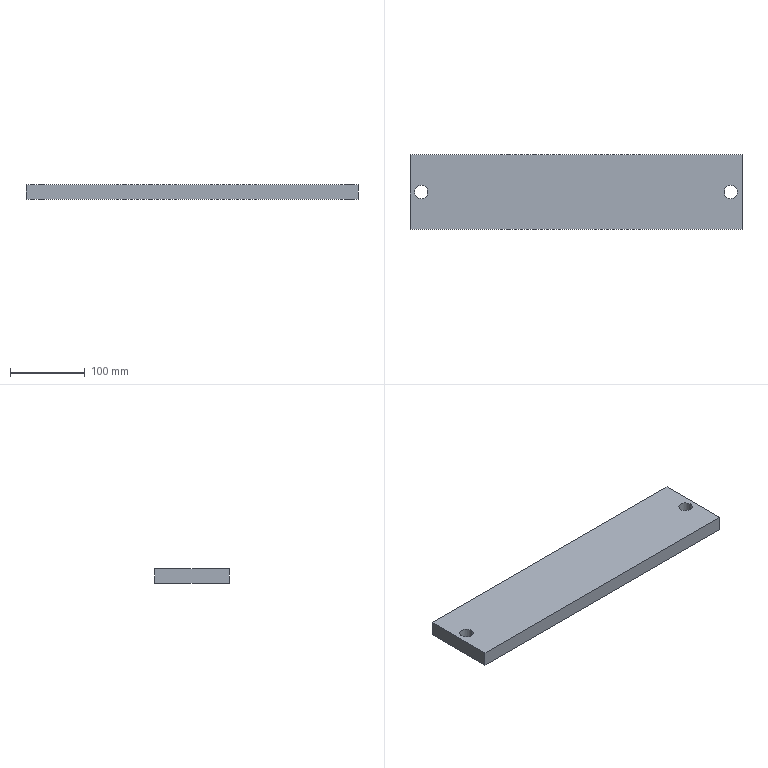Part | SolidWorks | features Extrusion 1 | 1 solid | 10 faces | box 445 x 100 x 20 mm | volume 879821 mm3 | plane 6 | cylinder 4 | commonest cylinder face diameters 18 x4
STEP:
#1=CARTESIAN_POINT('',(421.,50.,20.));
#2=VERTEX_POINT('',#1);
#3=CARTESIAN_POINT('',(439.,50.,20.));
#4=VERTEX_POINT('',#3);
#5=CARTESIAN_POINT('',(430.,50.,20.));
#6=DIRECTION('',(0.,0.,1.));
#7=DIRECTION('',(-1.,0.,0.));
#8=AXIS2_PLACEMENT_3D('',#5,#6,#7);
#9=CIRCLE('',#8,9.);
#10=EDGE_CURVE('',#2,#4,#9,.T.);
#11=ORIENTED_EDGE('',*,*,#10,.T.);
#12=CARTESIAN_POINT('',(439.,50.,0.));
#13=VERTEX_POINT('',#12);
#14=CARTESIAN_POINT('',(439.,50.,20.));
#15=DIRECTION('',(0.,0.,-1.));
#16=VECTOR('',#15,1000.);
#17=LINE('',#14,#16);
#18=EDGE_CURVE('',#4,#13,#17,.T.);
#19=ORIENTED_EDGE('',*,*,#18,.T.);
#20=CARTESIAN_POINT('',(421.,50.,0.));
#21=VERTEX_POINT('',#20);
#22=CARTESIAN_POINT('',(430.,50.,0.));
#23=DIRECTION('',(0.,0.,1.));
#24=DIRECTION('',(-1.,0.,0.));
#25=AXIS2_PLACEMENT_3D('',#22,#23,#24);
#26=CIRCLE('',#25,9.);
#27=EDGE_CURVE('',#21,#13,#26,.T.);
#28=ORIENTED_EDGE('',*,*,#27,.F.);
#29=CARTESIAN_POINT('',(421.,50.,20.));
#30=DIRECTION('',(0.,0.,-1.));
#31=VECTOR('',#30,1000.);
#32=LINE('',#29,#31);
#33=EDGE_CURVE('',#2,#21,#32,.T.);
#34=ORIENTED_EDGE('',*,*,#33,.F.);
#35=EDGE_LOOP('',(#11,#19,#28,#34));
#36=FACE_OUTER_BOUND('',#35,.T.);
#37=CARTESIAN_POINT('',(430.,50.,20.));
#38=DIRECTION('',(0.,0.,-1.));
#39=DIRECTION('',(-1.,0.,0.));
#40=AXIS2_PLACEMENT_3D('',#37,#38,#39);
#41=CYLINDRICAL_SURFACE('',#40,9.);
#42=ADVANCED_FACE('',(#36),#41,.F.);
#43=CARTESIAN_POINT('',(6.,50.,20.));
#44=VERTEX_POINT('',#43);
#45=CARTESIAN_POINT('',(24.,50.,20.));
#46=VERTEX_POINT('',#45);
#47=CARTESIAN_POINT('',(15.,50.,20.));
#48=DIRECTION('',(0.,0.,1.));
#49=DIRECTION('',(1.,0.,0.));
#50=AXIS2_PLACEMENT_3D('',#47,#48,#49);
#51=CIRCLE('',#50,9.);
#52=EDGE_CURVE('',#44,#46,#51,.T.);
#53=ORIENTED_EDGE('',*,*,#52,.T.);
#54=CARTESIAN_POINT('',(24.,50.,0.));
#55=VERTEX_POINT('',#54);
#56=CARTESIAN_POINT('',(24.,50.,20.));
#57=DIRECTION('',(0.,0.,-1.));
#58=VECTOR('',#57,1000.);
#59=LINE('',#56,#58);
#60=EDGE_CURVE('',#46,#55,#59,.T.);
#61=ORIENTED_EDGE('',*,*,#60,.T.);
#62=CARTESIAN_POINT('',(6.,50.,0.));
#63=VERTEX_POINT('',#62);
#64=CARTESIAN_POINT('',(15.,50.,0.));
#65=DIRECTION('',(0.,0.,1.));
#66=DIRECTION('',(1.,0.,0.));
#67=AXIS2_PLACEMENT_3D('',#64,#65,#66);
#68=CIRCLE('',#67,9.);
#69=EDGE_CURVE('',#63,#55,#68,.T.);
#70=ORIENTED_EDGE('',*,*,#69,.F.);
#71=CARTESIAN_POINT('',(6.,50.,20.));
#72=DIRECTION('',(0.,0.,-1.));
#73=VECTOR('',#72,1000.);
#74=LINE('',#71,#73);
#75=EDGE_CURVE('',#44,#63,#74,.T.);
#76=ORIENTED_EDGE('',*,*,#75,.F.);
#77=EDGE_LOOP('',(#53,#61,#70,#76));
#78=FACE_OUTER_BOUND('',#77,.T.);
#79=CARTESIAN_POINT('',(15.,50.,20.));
#80=DIRECTION('',(0.,0.,-1.));
#81=DIRECTION('',(-1.,0.,0.));
#82=AXIS2_PLACEMENT_3D('',#79,#80,#81);
#83=CYLINDRICAL_SURFACE('',#82,9.);
#84=ADVANCED_FACE('',(#78),#83,.F.);
#85=CARTESIAN_POINT('',(0.,100.,20.));
#86=VERTEX_POINT('',#85);
#87=CARTESIAN_POINT('',(0.,0.,20.));
#88=VERTEX_POINT('',#87);
#89=CARTESIAN_POINT('',(0.,0.,20.));
#90=DIRECTION('',(0.,-1.,0.));
#91=VECTOR('',#90,1000.);
#92=LINE('',#89,#91);
#93=EDGE_CURVE('',#86,#88,#92,.T.);
#94=ORIENTED_EDGE('',*,*,#93,.T.);
#95=CARTESIAN_POINT('',(445.,0.,20.));
#96=VERTEX_POINT('',#95);
#97=CARTESIAN_POINT('',(0.,0.,20.));
#98=DIRECTION('',(1.,0.,0.));
#99=VECTOR('',#98,1000.);
#100=LINE('',#97,#99);
#101=EDGE_CURVE('',#88,#96,#100,.T.);
#102=ORIENTED_EDGE('',*,*,#101,.T.);
#103=CARTESIAN_POINT('',(445.,100.,20.));
#104=VERTEX_POINT('',#103);
#105=CARTESIAN_POINT('',(445.,0.,20.));
#106=DIRECTION('',(0.,1.,0.));
#107=VECTOR('',#106,1000.);
#108=LINE('',#105,#107);
#109=EDGE_CURVE('',#96,#104,#108,.T.);
#110=ORIENTED_EDGE('',*,*,#109,.T.);
#111=CARTESIAN_POINT('',(0.,100.,20.));
#112=DIRECTION('',(-1.,0.,0.));
#113=VECTOR('',#112,1000.);
#114=LINE('',#111,#113);
#115=EDGE_CURVE('',#104,#86,#114,.T.);
#116=ORIENTED_EDGE('',*,*,#115,.T.);
#117=EDGE_LOOP('',(#94,#102,#110,#116));
#118=FACE_OUTER_BOUND('',#117,.T.);
#119=ORIENTED_EDGE('',*,*,#52,.F.);
#120=CARTESIAN_POINT('',(15.,50.,20.));
#121=DIRECTION('',(0.,0.,1.));
#122=DIRECTION('',(1.,0.,0.));
#123=AXIS2_PLACEMENT_3D('',#120,#121,#122);
#124=CIRCLE('',#123,9.);
#125=EDGE_CURVE('',#46,#44,#124,.T.);
#126=ORIENTED_EDGE('',*,*,#125,.F.);
#127=EDGE_LOOP('',(#119,#126));
#128=FACE_BOUND('',#127,.T.);
#129=ORIENTED_EDGE('',*,*,#10,.F.);
#130=CARTESIAN_POINT('',(430.,50.,20.));
#131=DIRECTION('',(0.,0.,1.));
#132=DIRECTION('',(-1.,0.,0.));
#133=AXIS2_PLACEMENT_3D('',#130,#131,#132);
#134=CIRCLE('',#133,9.);
#135=EDGE_CURVE('',#4,#2,#134,.T.);
#136=ORIENTED_EDGE('',*,*,#135,.F.);
#137=EDGE_LOOP('',(#129,#136));
#138=FACE_BOUND('',#137,.T.);
#139=CARTESIAN_POINT('',(0.,0.,20.));
#140=DIRECTION('',(0.,0.,-1.));
#141=DIRECTION('',(-1.,0.,0.));
#142=AXIS2_PLACEMENT_3D('',#139,#140,#141);
#143=PLANE('',#142);
#144=ADVANCED_FACE('',(#118,#128,#138),#143,.F.);
#145=ORIENTED_EDGE('',*,*,#69,.T.);
#146=CARTESIAN_POINT('',(15.,50.,0.));
#147=DIRECTION('',(0.,0.,1.));
#148=DIRECTION('',(1.,0.,0.));
#149=AXIS2_PLACEMENT_3D('',#146,#147,#148);
#150=CIRCLE('',#149,9.);
#151=EDGE_CURVE('',#55,#63,#150,.T.);
#152=ORIENTED_EDGE('',*,*,#151,.T.);
#153=EDGE_LOOP('',(#145,#152));
#154=FACE_BOUND('',#153,.T.);
#155=CARTESIAN_POINT('',(0.,100.,0.));
#156=VERTEX_POINT('',#155);
#157=CARTESIAN_POINT('',(0.,0.,0.));
#158=VERTEX_POINT('',#157);
#159=CARTESIAN_POINT('',(0.,0.,0.));
#160=DIRECTION('',(0.,-1.,0.));
#161=VECTOR('',#160,1000.);
#162=LINE('',#159,#161);
#163=EDGE_CURVE('',#156,#158,#162,.T.);
#164=ORIENTED_EDGE('',*,*,#163,.F.);
#165=CARTESIAN_POINT('',(445.,100.,0.));
#166=VERTEX_POINT('',#165);
#167=CARTESIAN_POINT('',(0.,100.,0.));
#168=DIRECTION('',(-1.,0.,0.));
#169=VECTOR('',#168,1000.);
#170=LINE('',#167,#169);
#171=EDGE_CURVE('',#166,#156,#170,.T.);
#172=ORIENTED_EDGE('',*,*,#171,.F.);
#173=CARTESIAN_POINT('',(445.,0.,0.));
#174=VERTEX_POINT('',#173);
#175=CARTESIAN_POINT('',(445.,0.,0.));
#176=DIRECTION('',(0.,1.,0.));
#177=VECTOR('',#176,1000.);
#178=LINE('',#175,#177);
#179=EDGE_CURVE('',#174,#166,#178,.T.);
#180=ORIENTED_EDGE('',*,*,#179,.F.);
#181=CARTESIAN_POINT('',(0.,0.,0.));
#182=DIRECTION('',(1.,0.,0.));
#183=VECTOR('',#182,1000.);
#184=LINE('',#181,#183);
#185=EDGE_CURVE('',#158,#174,#184,.T.);
#186=ORIENTED_EDGE('',*,*,#185,.F.);
#187=EDGE_LOOP('',(#164,#172,#180,#186));
#188=FACE_OUTER_BOUND('',#187,.T.);
#189=ORIENTED_EDGE('',*,*,#27,.T.);
#190=CARTESIAN_POINT('',(430.,50.,0.));
#191=DIRECTION('',(0.,0.,1.));
#192=DIRECTION('',(-1.,0.,0.));
#193=AXIS2_PLACEMENT_3D('',#190,#191,#192);
#194=CIRCLE('',#193,9.);
#195=EDGE_CURVE('',#13,#21,#194,.T.);
#196=ORIENTED_EDGE('',*,*,#195,.T.);
#197=EDGE_LOOP('',(#189,#196));
#198=FACE_BOUND('',#197,.T.);
#199=CARTESIAN_POINT('',(0.,0.,0.));
#200=DIRECTION('',(0.,0.,-1.));
#201=DIRECTION('',(-1.,0.,0.));
#202=AXIS2_PLACEMENT_3D('',#199,#200,#201);
#203=PLANE('',#202);
#204=ADVANCED_FACE('',(#154,#188,#198),#203,.T.);
#205=ORIENTED_EDGE('',*,*,#163,.T.);
#206=CARTESIAN_POINT('',(0.,0.,20.));
#207=DIRECTION('',(0.,0.,-1.));
#208=VECTOR('',#207,1000.);
#209=LINE('',#206,#208);
#210=EDGE_CURVE('',#88,#158,#209,.T.);
#211=ORIENTED_EDGE('',*,*,#210,.F.);
#212=ORIENTED_EDGE('',*,*,#93,.F.);
#213=CARTESIAN_POINT('',(0.,100.,20.));
#214=DIRECTION('',(0.,0.,-1.));
#215=VECTOR('',#214,1000.);
#216=LINE('',#213,#215);
#217=EDGE_CURVE('',#86,#156,#216,.T.);
#218=ORIENTED_EDGE('',*,*,#217,.T.);
#219=EDGE_LOOP('',(#205,#211,#212,#218));
#220=FACE_OUTER_BOUND('',#219,.T.);
#221=CARTESIAN_POINT('',(0.,0.,20.));
#222=DIRECTION('',(1.,0.,0.));
#223=DIRECTION('',(0.,0.,-1.));
#224=AXIS2_PLACEMENT_3D('',#221,#222,#223);
#225=PLANE('',#224);
#226=ADVANCED_FACE('',(#220),#225,.F.);
#227=ORIENTED_EDGE('',*,*,#185,.T.);
#228=CARTESIAN_POINT('',(445.,0.,20.));
#229=DIRECTION('',(0.,0.,-1.));
#230=VECTOR('',#229,1000.);
#231=LINE('',#228,#230);
#232=EDGE_CURVE('',#96,#174,#231,.T.);
#233=ORIENTED_EDGE('',*,*,#232,.F.);
#234=ORIENTED_EDGE('',*,*,#101,.F.);
#235=ORIENTED_EDGE('',*,*,#210,.T.);
#236=EDGE_LOOP('',(#227,#233,#234,#235));
#237=FACE_OUTER_BOUND('',#236,.T.);
#238=CARTESIAN_POINT('',(0.,0.,20.));
#239=DIRECTION('',(0.,1.,0.));
#240=DIRECTION('',(0.,0.,1.));
#241=AXIS2_PLACEMENT_3D('',#238,#239,#240);
#242=PLANE('',#241);
#243=ADVANCED_FACE('',(#237),#242,.F.);
#244=ORIENTED_EDGE('',*,*,#179,.T.);
#245=CARTESIAN_POINT('',(445.,100.,20.));
#246=DIRECTION('',(0.,0.,-1.));
#247=VECTOR('',#246,1000.);
#248=LINE('',#245,#247);
#249=EDGE_CURVE('',#104,#166,#248,.T.);
#250=ORIENTED_EDGE('',*,*,#249,.F.);
#251=ORIENTED_EDGE('',*,*,#109,.F.);
#252=ORIENTED_EDGE('',*,*,#232,.T.);
#253=EDGE_LOOP('',(#244,#250,#251,#252));
#254=FACE_OUTER_BOUND('',#253,.T.);
#255=CARTESIAN_POINT('',(445.,0.,20.));
#256=DIRECTION('',(-1.,0.,0.));
#257=DIRECTION('',(0.,0.,1.));
#258=AXIS2_PLACEMENT_3D('',#255,#256,#257);
#259=PLANE('',#258);
#260=ADVANCED_FACE('',(#254),#259,.F.);
#261=ORIENTED_EDGE('',*,*,#171,.T.);
#262=ORIENTED_EDGE('',*,*,#217,.F.);
#263=ORIENTED_EDGE('',*,*,#115,.F.);
#264=ORIENTED_EDGE('',*,*,#249,.T.);
#265=EDGE_LOOP('',(#261,#262,#263,#264));
#266=FACE_OUTER_BOUND('',#265,.T.);
#267=CARTESIAN_POINT('',(0.,100.,20.));
#268=DIRECTION('',(0.,-1.,0.));
#269=DIRECTION('',(0.,0.,-1.));
#270=AXIS2_PLACEMENT_3D('',#267,#268,#269);
#271=PLANE('',#270);
#272=ADVANCED_FACE('',(#266),#271,.F.);
#273=ORIENTED_EDGE('',*,*,#60,.F.);
#274=ORIENTED_EDGE('',*,*,#125,.T.);
#275=ORIENTED_EDGE('',*,*,#75,.T.);
#276=ORIENTED_EDGE('',*,*,#151,.F.);
#277=EDGE_LOOP('',(#273,#274,#275,#276));
#278=FACE_OUTER_BOUND('',#277,.T.);
#279=CARTESIAN_POINT('',(15.,50.,20.));
#280=DIRECTION('',(0.,0.,-1.));
#281=DIRECTION('',(-1.,0.,0.));
#282=AXIS2_PLACEMENT_3D('',#279,#280,#281);
#283=CYLINDRICAL_SURFACE('',#282,9.);
#284=ADVANCED_FACE('',(#278),#283,.F.);
#285=ORIENTED_EDGE('',*,*,#18,.F.);
#286=ORIENTED_EDGE('',*,*,#135,.T.);
#287=ORIENTED_EDGE('',*,*,#33,.T.);
#288=ORIENTED_EDGE('',*,*,#195,.F.);
#289=EDGE_LOOP('',(#285,#286,#287,#288));
#290=FACE_OUTER_BOUND('',#289,.T.);
#291=CARTESIAN_POINT('',(430.,50.,20.));
#292=DIRECTION('',(0.,0.,-1.));
#293=DIRECTION('',(-1.,0.,0.));
#294=AXIS2_PLACEMENT_3D('',#291,#292,#293);
#295=CYLINDRICAL_SURFACE('',#294,9.);
#296=ADVANCED_FACE('',(#290),#295,.F.);
#297=CLOSED_SHELL('',(#42,#84,#144,#204,#226,#243,#260,#272,#284,#296));
#298=MANIFOLD_SOLID_BREP('',#297);
#299=CARTESIAN_POINT('',(0.,0.,0.));
#300=DIRECTION('',(0.,0.,1.));
#301=DIRECTION('',(1.,0.,0.));
#302=AXIS2_PLACEMENT_3D('',#299,#300,#301);
#303=(LENGTH_UNIT()NAMED_UNIT(*)SI_UNIT(.MILLI.,.METRE.));
#304=UNCERTAINTY_MEASURE_WITH_UNIT(LENGTH_MEASURE(0.00001),#303,'','');
#305=(NAMED_UNIT(*)PLANE_ANGLE_UNIT()SI_UNIT($,.RADIAN.));
#306=(NAMED_UNIT(*)SI_UNIT($,.STERADIAN.)SOLID_ANGLE_UNIT());
#307=(GEOMETRIC_REPRESENTATION_CONTEXT(3)GLOBAL_UNCERTAINTY_ASSIGNED_CONTEXT((#304))GLOBAL_UNIT_ASSIGNED_CONTEXT((#303,#305,#306))REPRESENTATION_CONTEXT('',''));
#308=ADVANCED_BREP_SHAPE_REPRESENTATION('',(#298,#302),#307);